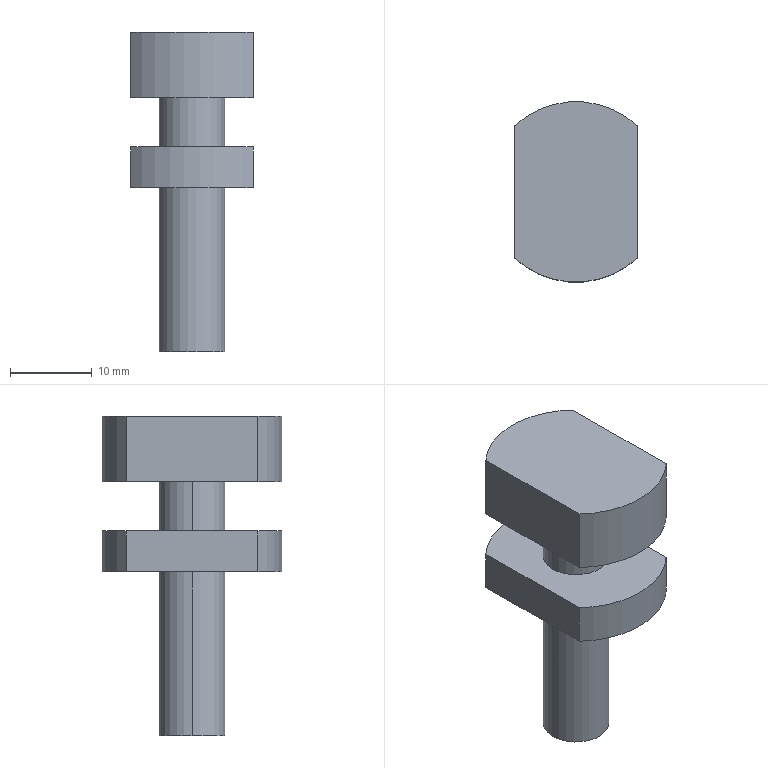Part | STEP file | iron shell displacement union | 1 solid | 17 faces | box 15 x 22 x 39 mm | volume 5236 mm3 | plane 9 | cylinder 8 | commonest cylinder face diameters 8 x4 22 x4
STEP:
#1=CARTESIAN_POINT('',(0.,0.,0.));
#2=DIRECTION('',(0.,0.,1.));
#3=DIRECTION('',(1.,0.,0.));
#4=AXIS2_PLACEMENT_3D('',#1,#2,#3);
#5=CARTESIAN_POINT('',(4.,0.,0.));
#6=VERTEX_POINT('',#5);
#7=CARTESIAN_POINT('',(-4.,0.,0.));
#8=VERTEX_POINT('',#7);
#9=CARTESIAN_POINT('',(0.,0.,0.));
#10=DIRECTION('',(0.,0.,1.));
#11=DIRECTION('',(1.,0.,0.));
#12=AXIS2_PLACEMENT_3D('',#9,#10,#11);
#13=CIRCLE('',#12,4.);
#14=CARTESIAN_POINT('',(0.,0.,39.));
#15=DIRECTION('',(0.,0.,1.));
#16=DIRECTION('',(1.,0.,0.));
#17=AXIS2_PLACEMENT_3D('',#14,#15,#16);
#18=CYLINDRICAL_SURFACE('',#17,4.);
#19=CARTESIAN_POINT('',(0.,-39.));
#20=DIRECTION('',(1.,0.));
#21=VECTOR('',#20,1.);
#22=LINE('',#19,#21);
#23=(GEOMETRIC_REPRESENTATION_CONTEXT(2)PARAMETRIC_REPRESENTATION_CONTEXT()REPRESENTATION_CONTEXT('',''));
#24=DEFINITIONAL_REPRESENTATION('',(#22),#23);
#25=PCURVE('',#18,#24);
#26=CARTESIAN_POINT('',(0.,0.,0.));
#27=DIRECTION('',(0.,0.,1.));
#28=DIRECTION('',(1.,0.,0.));
#29=AXIS2_PLACEMENT_3D('',#26,#27,#28);
#30=PLANE('',#29);
#31=CARTESIAN_POINT('',(0.,0.));
#32=DIRECTION('',(1.,0.));
#33=AXIS2_PLACEMENT_2D('',#31,#32);
#34=CIRCLE('',#33,4.);
#35=(GEOMETRIC_REPRESENTATION_CONTEXT(2)PARAMETRIC_REPRESENTATION_CONTEXT()REPRESENTATION_CONTEXT('',''));
#36=DEFINITIONAL_REPRESENTATION('',(#34),#35);
#37=PCURVE('',#30,#36);
#38=SURFACE_CURVE('',#13,(#25,#37),.PCURVE_S1.);
#39=EDGE_CURVE('',#6,#8,#38,.T.);
#40=ORIENTED_EDGE('',*,*,#39,.T.);
#41=CARTESIAN_POINT('',(-4.,0.,20.));
#42=VERTEX_POINT('',#41);
#43=CARTESIAN_POINT('',(-4.,0.,39.));
#44=DIRECTION('',(0.,0.,1.));
#45=VECTOR('',#44,1.);
#46=LINE('',#43,#45);
#47=CARTESIAN_POINT('',(3.142,0.));
#48=DIRECTION('',(0.,1.));
#49=VECTOR('',#48,1.);
#50=LINE('',#47,#49);
#51=(GEOMETRIC_REPRESENTATION_CONTEXT(2)PARAMETRIC_REPRESENTATION_CONTEXT()REPRESENTATION_CONTEXT('',''));
#52=DEFINITIONAL_REPRESENTATION('',(#50),#51);
#53=PCURVE('',#18,#52);
#54=CARTESIAN_POINT('',(0.,0.,39.));
#55=DIRECTION('',(0.,0.,1.));
#56=DIRECTION('',(1.,0.,0.));
#57=AXIS2_PLACEMENT_3D('',#54,#55,#56);
#58=CYLINDRICAL_SURFACE('',#57,4.);
#59=CARTESIAN_POINT('',(3.142,0.));
#60=DIRECTION('',(0.,1.));
#61=VECTOR('',#60,1.);
#62=LINE('',#59,#61);
#63=(GEOMETRIC_REPRESENTATION_CONTEXT(2)PARAMETRIC_REPRESENTATION_CONTEXT()REPRESENTATION_CONTEXT('',''));
#64=DEFINITIONAL_REPRESENTATION('',(#62),#63);
#65=PCURVE('',#58,#64);
#66=SURFACE_CURVE('',#46,(#53,#65),.PCURVE_S1.);
#67=EDGE_CURVE('',#8,#42,#66,.T.);
#68=ORIENTED_EDGE('',*,*,#67,.T.);
#69=CARTESIAN_POINT('',(4.,0.,20.));
#70=VERTEX_POINT('',#69);
#71=CARTESIAN_POINT('',(0.,0.,20.));
#72=DIRECTION('',(0.,0.,1.));
#73=DIRECTION('',(1.,0.,0.));
#74=AXIS2_PLACEMENT_3D('',#71,#72,#73);
#75=CIRCLE('',#74,4.);
#76=CARTESIAN_POINT('',(0.,-19.));
#77=DIRECTION('',(1.,0.));
#78=VECTOR('',#77,1.);
#79=LINE('',#76,#78);
#80=(GEOMETRIC_REPRESENTATION_CONTEXT(2)PARAMETRIC_REPRESENTATION_CONTEXT()REPRESENTATION_CONTEXT('',''));
#81=DEFINITIONAL_REPRESENTATION('',(#79),#80);
#82=PCURVE('',#18,#81);
#83=CARTESIAN_POINT('',(-4.,0.,20.));
#84=DIRECTION('',(0.,0.,-1.));
#85=DIRECTION('',(-1.,0.,0.));
#86=AXIS2_PLACEMENT_3D('',#83,#84,#85);
#87=PLANE('',#86);
#88=CARTESIAN_POINT('',(-8.,0.));
#89=CARTESIAN_POINT('',(-8.,6.928));
#90=CARTESIAN_POINT('',(-2.,3.464));
#91=CARTESIAN_POINT('',(4.,0.));
#92=CARTESIAN_POINT('',(-2.,-3.464));
#93=CARTESIAN_POINT('',(-8.,-6.928));
#94=CARTESIAN_POINT('',(-8.,0.));
#95=(BOUNDED_CURVE()B_SPLINE_CURVE(2,(#88,#89,#90,#91,#92,#93,#94),.UNSPECIFIED.,.T.,.F.)B_SPLINE_CURVE_WITH_KNOTS((1,2,2,2,2,1),(-2.094,0.,2.094,4.189,6.283,8.378),.UNSPECIFIED.)CURVE()GEOMETRIC_REPRESENTATION_ITEM()RATIONAL_B_SPLINE_CURVE((1.,0.5,1.,0.5,1.,0.5,1.))REPRESENTATION_ITEM(''));
#96=(GEOMETRIC_REPRESENTATION_CONTEXT(2)PARAMETRIC_REPRESENTATION_CONTEXT()REPRESENTATION_CONTEXT('',''));
#97=DEFINITIONAL_REPRESENTATION('',(#95),#96);
#98=PCURVE('',#87,#97);
#99=SURFACE_CURVE('',#75,(#82,#98),.PCURVE_S1.);
#100=EDGE_CURVE('',#70,#42,#99,.T.);
#101=ORIENTED_EDGE('',*,*,#100,.F.);
#102=CARTESIAN_POINT('',(4.,0.,39.));
#103=DIRECTION('',(0.,0.,1.));
#104=VECTOR('',#103,1.);
#105=LINE('',#102,#104);
#106=CARTESIAN_POINT('',(0.,0.));
#107=DIRECTION('',(0.,1.));
#108=VECTOR('',#107,1.);
#109=LINE('',#106,#108);
#110=(GEOMETRIC_REPRESENTATION_CONTEXT(2)PARAMETRIC_REPRESENTATION_CONTEXT()REPRESENTATION_CONTEXT('',''));
#111=DEFINITIONAL_REPRESENTATION('',(#109),#110);
#112=PCURVE('',#18,#111);
#113=CARTESIAN_POINT('',(6.283,0.));
#114=DIRECTION('',(0.,1.));
#115=VECTOR('',#114,1.);
#116=LINE('',#113,#115);
#117=(GEOMETRIC_REPRESENTATION_CONTEXT(2)PARAMETRIC_REPRESENTATION_CONTEXT()REPRESENTATION_CONTEXT('',''));
#118=DEFINITIONAL_REPRESENTATION('',(#116),#117);
#119=PCURVE('',#58,#118);
#120=SURFACE_CURVE('',#105,(#112,#119),.PCURVE_S1.);
#121=EDGE_CURVE('',#6,#70,#120,.T.);
#122=ORIENTED_EDGE('',*,*,#121,.F.);
#123=EDGE_LOOP('',(#40,#68,#101,#122));
#124=FACE_BOUND('',#123,.T.);
#125=ADVANCED_FACE('',(#124),#18,.T.);
#126=CARTESIAN_POINT('',(4.,0.,25.));
#127=VERTEX_POINT('',#126);
#128=CARTESIAN_POINT('',(-4.,0.,25.));
#129=VERTEX_POINT('',#128);
#130=CARTESIAN_POINT('',(0.,0.,25.));
#131=DIRECTION('',(0.,0.,1.));
#132=DIRECTION('',(1.,0.,0.));
#133=AXIS2_PLACEMENT_3D('',#130,#131,#132);
#134=CIRCLE('',#133,4.);
#135=CARTESIAN_POINT('',(0.,0.,39.));
#136=DIRECTION('',(0.,0.,1.));
#137=DIRECTION('',(1.,0.,0.));
#138=AXIS2_PLACEMENT_3D('',#135,#136,#137);
#139=CYLINDRICAL_SURFACE('',#138,4.);
#140=CARTESIAN_POINT('',(0.,-14.));
#141=DIRECTION('',(1.,0.));
#142=VECTOR('',#141,1.);
#143=LINE('',#140,#142);
#144=(GEOMETRIC_REPRESENTATION_CONTEXT(2)PARAMETRIC_REPRESENTATION_CONTEXT()REPRESENTATION_CONTEXT('',''));
#145=DEFINITIONAL_REPRESENTATION('',(#143),#144);
#146=PCURVE('',#139,#145);
#147=CARTESIAN_POINT('',(-18.905,0.,25.));
#148=DIRECTION('',(0.,0.,1.));
#149=DIRECTION('',(1.,0.,0.));
#150=AXIS2_PLACEMENT_3D('',#147,#148,#149);
#151=PLANE('',#150);
#152=CARTESIAN_POINT('',(18.905,0.));
#153=DIRECTION('',(1.,0.));
#154=AXIS2_PLACEMENT_2D('',#152,#153);
#155=CIRCLE('',#154,4.);
#156=(GEOMETRIC_REPRESENTATION_CONTEXT(2)PARAMETRIC_REPRESENTATION_CONTEXT()REPRESENTATION_CONTEXT('',''));
#157=DEFINITIONAL_REPRESENTATION('',(#155),#156);
#158=PCURVE('',#151,#157);
#159=SURFACE_CURVE('',#134,(#146,#158),.PCURVE_S1.);
#160=EDGE_CURVE('',#127,#129,#159,.T.);
#161=ORIENTED_EDGE('',*,*,#160,.T.);
#162=CARTESIAN_POINT('',(-4.,0.,31.));
#163=VERTEX_POINT('',#162);
#164=CARTESIAN_POINT('',(-4.,0.,39.));
#165=DIRECTION('',(0.,0.,1.));
#166=VECTOR('',#165,1.);
#167=LINE('',#164,#166);
#168=CARTESIAN_POINT('',(3.142,0.));
#169=DIRECTION('',(0.,1.));
#170=VECTOR('',#169,1.);
#171=LINE('',#168,#170);
#172=(GEOMETRIC_REPRESENTATION_CONTEXT(2)PARAMETRIC_REPRESENTATION_CONTEXT()REPRESENTATION_CONTEXT('',''));
#173=DEFINITIONAL_REPRESENTATION('',(#171),#172);
#174=PCURVE('',#139,#173);
#175=CARTESIAN_POINT('',(0.,0.,39.));
#176=DIRECTION('',(0.,0.,1.));
#177=DIRECTION('',(1.,0.,0.));
#178=AXIS2_PLACEMENT_3D('',#175,#176,#177);
#179=CYLINDRICAL_SURFACE('',#178,4.);
#180=CARTESIAN_POINT('',(3.142,0.));
#181=DIRECTION('',(0.,1.));
#182=VECTOR('',#181,1.);
#183=LINE('',#180,#182);
#184=(GEOMETRIC_REPRESENTATION_CONTEXT(2)PARAMETRIC_REPRESENTATION_CONTEXT()REPRESENTATION_CONTEXT('',''));
#185=DEFINITIONAL_REPRESENTATION('',(#183),#184);
#186=PCURVE('',#179,#185);
#187=SURFACE_CURVE('',#167,(#174,#186),.PCURVE_S1.);
#188=EDGE_CURVE('',#129,#163,#187,.T.);
#189=ORIENTED_EDGE('',*,*,#188,.T.);
#190=CARTESIAN_POINT('',(4.,0.,31.));
#191=VERTEX_POINT('',#190);
#192=CARTESIAN_POINT('',(0.,0.,31.));
#193=DIRECTION('',(0.,0.,1.));
#194=DIRECTION('',(1.,0.,0.));
#195=AXIS2_PLACEMENT_3D('',#192,#193,#194);
#196=CIRCLE('',#195,4.);
#197=CARTESIAN_POINT('',(0.,-8.));
#198=DIRECTION('',(1.,0.));
#199=VECTOR('',#198,1.);
#200=LINE('',#197,#199);
#201=(GEOMETRIC_REPRESENTATION_CONTEXT(2)PARAMETRIC_REPRESENTATION_CONTEXT()REPRESENTATION_CONTEXT('',''));
#202=DEFINITIONAL_REPRESENTATION('',(#200),#201);
#203=PCURVE('',#139,#202);
#204=CARTESIAN_POINT('',(-18.905,0.,31.));
#205=DIRECTION('',(0.,0.,-1.));
#206=DIRECTION('',(-1.,0.,0.));
#207=AXIS2_PLACEMENT_3D('',#204,#205,#206);
#208=PLANE('',#207);
#209=CARTESIAN_POINT('',(-22.905,0.));
#210=CARTESIAN_POINT('',(-22.905,6.928));
#211=CARTESIAN_POINT('',(-16.905,3.464));
#212=CARTESIAN_POINT('',(-10.905,0.));
#213=CARTESIAN_POINT('',(-16.905,-3.464));
#214=CARTESIAN_POINT('',(-22.905,-6.928));
#215=CARTESIAN_POINT('',(-22.905,0.));
#216=(BOUNDED_CURVE()B_SPLINE_CURVE(2,(#209,#210,#211,#212,#213,#214,#215),.UNSPECIFIED.,.T.,.F.)B_SPLINE_CURVE_WITH_KNOTS((1,2,2,2,2,1),(-2.094,0.,2.094,4.189,6.283,8.378),.UNSPECIFIED.)CURVE()GEOMETRIC_REPRESENTATION_ITEM()RATIONAL_B_SPLINE_CURVE((1.,0.5,1.,0.5,1.,0.5,1.))REPRESENTATION_ITEM(''));
#217=(GEOMETRIC_REPRESENTATION_CONTEXT(2)PARAMETRIC_REPRESENTATION_CONTEXT()REPRESENTATION_CONTEXT('',''));
#218=DEFINITIONAL_REPRESENTATION('',(#216),#217);
#219=PCURVE('',#208,#218);
#220=SURFACE_CURVE('',#196,(#203,#219),.PCURVE_S1.);
#221=EDGE_CURVE('',#191,#163,#220,.T.);
#222=ORIENTED_EDGE('',*,*,#221,.F.);
#223=CARTESIAN_POINT('',(4.,0.,39.));
#224=DIRECTION('',(0.,0.,1.));
#225=VECTOR('',#224,1.);
#226=LINE('',#223,#225);
#227=CARTESIAN_POINT('',(0.,0.));
#228=DIRECTION('',(0.,1.));
#229=VECTOR('',#228,1.);
#230=LINE('',#227,#229);
#231=(GEOMETRIC_REPRESENTATION_CONTEXT(2)PARAMETRIC_REPRESENTATION_CONTEXT()REPRESENTATION_CONTEXT('',''));
#232=DEFINITIONAL_REPRESENTATION('',(#230),#231);
#233=PCURVE('',#139,#232);
#234=CARTESIAN_POINT('',(6.283,0.));
#235=DIRECTION('',(0.,1.));
#236=VECTOR('',#235,1.);
#237=LINE('',#234,#236);
#238=(GEOMETRIC_REPRESENTATION_CONTEXT(2)PARAMETRIC_REPRESENTATION_CONTEXT()REPRESENTATION_CONTEXT('',''));
#239=DEFINITIONAL_REPRESENTATION('',(#237),#238);
#240=PCURVE('',#179,#239);
#241=SURFACE_CURVE('',#226,(#233,#240),.PCURVE_S1.);
#242=EDGE_CURVE('',#127,#191,#241,.T.);
#243=ORIENTED_EDGE('',*,*,#242,.F.);
#244=EDGE_LOOP('',(#161,#189,#222,#243));
#245=FACE_BOUND('',#244,.T.);
#246=ADVANCED_FACE('',(#245),#139,.T.);
#247=CARTESIAN_POINT('',(-7.5,-8.047,20.));
#248=VERTEX_POINT('',#247);
#249=CARTESIAN_POINT('',(-7.5,8.047,20.));
#250=VERTEX_POINT('',#249);
#251=CARTESIAN_POINT('',(-7.5,8.047,20.));
#252=DIRECTION('',(0.,1.,0.));
#253=VECTOR('',#252,1.);
#254=LINE('',#251,#253);
#255=CARTESIAN_POINT('',(-7.5,8.047,39.));
#256=DIRECTION('',(1.,0.,0.));
#257=DIRECTION('',(0.,0.,-1.));
#258=AXIS2_PLACEMENT_3D('',#255,#256,#257);
#259=PLANE('',#258);
#260=CARTESIAN_POINT('',(19.,0.));
#261=DIRECTION('',(0.,1.));
#262=VECTOR('',#261,1.);
#263=LINE('',#260,#262);
#264=(GEOMETRIC_REPRESENTATION_CONTEXT(2)PARAMETRIC_REPRESENTATION_CONTEXT()REPRESENTATION_CONTEXT('',''));
#265=DEFINITIONAL_REPRESENTATION('',(#263),#264);
#266=PCURVE('',#259,#265);
#267=CARTESIAN_POINT('',(3.5,8.047));
#268=DIRECTION('',(0.,1.));
#269=VECTOR('',#268,1.);
#270=LINE('',#267,#269);
#271=(GEOMETRIC_REPRESENTATION_CONTEXT(2)PARAMETRIC_REPRESENTATION_CONTEXT()REPRESENTATION_CONTEXT('',''));
#272=DEFINITIONAL_REPRESENTATION('',(#270),#271);
#273=PCURVE('',#87,#272);
#274=SURFACE_CURVE('',#254,(#266,#273),.PCURVE_S1.);
#275=EDGE_CURVE('',#248,#250,#274,.T.);
#276=ORIENTED_EDGE('',*,*,#275,.F.);
#277=CARTESIAN_POINT('',(-7.5,-8.047,25.));
#278=VERTEX_POINT('',#277);
#279=CARTESIAN_POINT('',(-7.5,-8.047,39.));
#280=DIRECTION('',(0.,0.,-1.));
#281=VECTOR('',#280,1.);
#282=LINE('',#279,#281);
#283=CARTESIAN_POINT('',(0.,-16.093));
#284=DIRECTION('',(1.,0.));
#285=VECTOR('',#284,1.);
#286=LINE('',#283,#285);
#287=(GEOMETRIC_REPRESENTATION_CONTEXT(2)PARAMETRIC_REPRESENTATION_CONTEXT()REPRESENTATION_CONTEXT('',''));
#288=DEFINITIONAL_REPRESENTATION('',(#286),#287);
#289=PCURVE('',#259,#288);
#290=CARTESIAN_POINT('',(0.,0.,39.));
#291=DIRECTION('',(0.,0.,-1.));
#292=DIRECTION('',(-1.,0.,0.));
#293=AXIS2_PLACEMENT_3D('',#290,#291,#292);
#294=CYLINDRICAL_SURFACE('',#293,11.);
#295=CARTESIAN_POINT('',(5.463,0.));
#296=DIRECTION('',(0.,1.));
#297=VECTOR('',#296,1.);
#298=LINE('',#295,#297);
#299=(GEOMETRIC_REPRESENTATION_CONTEXT(2)PARAMETRIC_REPRESENTATION_CONTEXT()REPRESENTATION_CONTEXT('',''));
#300=DEFINITIONAL_REPRESENTATION('',(#298),#299);
#301=PCURVE('',#294,#300);
#302=SURFACE_CURVE('',#282,(#289,#301),.PCURVE_S1.);
#303=EDGE_CURVE('',#278,#248,#302,.T.);
#304=ORIENTED_EDGE('',*,*,#303,.F.);
#305=CARTESIAN_POINT('',(-7.5,8.047,25.));
#306=VERTEX_POINT('',#305);
#307=CARTESIAN_POINT('',(-7.5,8.047,25.));
#308=DIRECTION('',(0.,-1.,0.));
#309=VECTOR('',#308,1.);
#310=LINE('',#307,#309);
#311=CARTESIAN_POINT('',(14.,0.));
#312=DIRECTION('',(0.,-1.));
#313=VECTOR('',#312,1.);
#314=LINE('',#311,#313);
#315=(GEOMETRIC_REPRESENTATION_CONTEXT(2)PARAMETRIC_REPRESENTATION_CONTEXT()REPRESENTATION_CONTEXT('',''));
#316=DEFINITIONAL_REPRESENTATION('',(#314),#315);
#317=PCURVE('',#259,#316);
#318=CARTESIAN_POINT('',(11.405,8.047));
#319=DIRECTION('',(0.,-1.));
#320=VECTOR('',#319,1.);
#321=LINE('',#318,#320);
#322=(GEOMETRIC_REPRESENTATION_CONTEXT(2)PARAMETRIC_REPRESENTATION_CONTEXT()REPRESENTATION_CONTEXT('',''));
#323=DEFINITIONAL_REPRESENTATION('',(#321),#322);
#324=PCURVE('',#151,#323);
#325=SURFACE_CURVE('',#310,(#317,#324),.PCURVE_S1.);
#326=EDGE_CURVE('',#306,#278,#325,.T.);
#327=ORIENTED_EDGE('',*,*,#326,.F.);
#328=CARTESIAN_POINT('',(-7.5,8.047,39.));
#329=DIRECTION('',(0.,0.,-1.));
#330=VECTOR('',#329,1.);
#331=LINE('',#328,#330);
#332=CARTESIAN_POINT('',(0.,0.));
#333=DIRECTION('',(1.,0.));
#334=VECTOR('',#333,1.);
#335=LINE('',#332,#334);
#336=(GEOMETRIC_REPRESENTATION_CONTEXT(2)PARAMETRIC_REPRESENTATION_CONTEXT()REPRESENTATION_CONTEXT('',''));
#337=DEFINITIONAL_REPRESENTATION('',(#335),#336);
#338=PCURVE('',#259,#337);
#339=CARTESIAN_POINT('',(0.,0.,39.));
#340=DIRECTION('',(0.,0.,-1.));
#341=DIRECTION('',(-1.,0.,0.));
#342=AXIS2_PLACEMENT_3D('',#339,#340,#341);
#343=CYLINDRICAL_SURFACE('',#342,11.);
#344=CARTESIAN_POINT('',(0.8206,0.));
#345=DIRECTION('',(0.,1.));
#346=VECTOR('',#345,1.);
#347=LINE('',#344,#346);
#348=(GEOMETRIC_REPRESENTATION_CONTEXT(2)PARAMETRIC_REPRESENTATION_CONTEXT()REPRESENTATION_CONTEXT('',''));
#349=DEFINITIONAL_REPRESENTATION('',(#347),#348);
#350=PCURVE('',#343,#349);
#351=SURFACE_CURVE('',#331,(#338,#350),.PCURVE_S1.);
#352=EDGE_CURVE('',#306,#250,#351,.T.);
#353=ORIENTED_EDGE('',*,*,#352,.T.);
#354=EDGE_LOOP('',(#276,#304,#327,#353));
#355=FACE_BOUND('',#354,.T.);
#356=ADVANCED_FACE('',(#355),#259,.F.);
#357=CARTESIAN_POINT('',(7.5,8.047,20.));
#358=VERTEX_POINT('',#357);
#359=CARTESIAN_POINT('',(0.,0.,20.));
#360=DIRECTION('',(0.,0.,-1.));
#361=DIRECTION('',(-1.,0.,0.));
#362=AXIS2_PLACEMENT_3D('',#359,#360,#361);
#363=CIRCLE('',#362,11.);
#364=CARTESIAN_POINT('',(0.,19.));
#365=DIRECTION('',(1.,0.));
#366=VECTOR('',#365,1.);
#367=LINE('',#364,#366);
#368=(GEOMETRIC_REPRESENTATION_CONTEXT(2)PARAMETRIC_REPRESENTATION_CONTEXT()REPRESENTATION_CONTEXT('',''));
#369=DEFINITIONAL_REPRESENTATION('',(#367),#368);
#370=PCURVE('',#343,#369);
#371=CARTESIAN_POINT('',(-4.,0.));
#372=DIRECTION('',(1.,0.));
#373=AXIS2_PLACEMENT_2D('',#371,#372);
#374=CIRCLE('',#373,11.);
#375=(GEOMETRIC_REPRESENTATION_CONTEXT(2)PARAMETRIC_REPRESENTATION_CONTEXT()REPRESENTATION_CONTEXT('',''));
#376=DEFINITIONAL_REPRESENTATION('',(#374),#375);
#377=PCURVE('',#87,#376);
#378=SURFACE_CURVE('',#363,(#370,#377),.PCURVE_S1.);
#379=EDGE_CURVE('',#250,#358,#378,.T.);
#380=ORIENTED_EDGE('',*,*,#379,.F.);
#381=ORIENTED_EDGE('',*,*,#352,.F.);
#382=CARTESIAN_POINT('',(7.5,8.047,25.));
#383=VERTEX_POINT('',#382);
#384=CARTESIAN_POINT('',(0.,0.,25.));
#385=DIRECTION('',(0.,0.,1.));
#386=DIRECTION('',(1.,0.,0.));
#387=AXIS2_PLACEMENT_3D('',#384,#385,#386);
#388=CIRCLE('',#387,11.);
#389=CARTESIAN_POINT('',(3.142,14.));
#390=DIRECTION('',(-1.,0.));
#391=VECTOR('',#390,1.);
#392=LINE('',#389,#391);
#393=(GEOMETRIC_REPRESENTATION_CONTEXT(2)PARAMETRIC_REPRESENTATION_CONTEXT()REPRESENTATION_CONTEXT('',''));
#394=DEFINITIONAL_REPRESENTATION('',(#392),#393);
#395=PCURVE('',#343,#394);
#396=CARTESIAN_POINT('',(18.905,0.));
#397=DIRECTION('',(1.,0.));
#398=AXIS2_PLACEMENT_2D('',#396,#397);
#399=CIRCLE('',#398,11.);
#400=(GEOMETRIC_REPRESENTATION_CONTEXT(2)PARAMETRIC_REPRESENTATION_CONTEXT()REPRESENTATION_CONTEXT('',''));
#401=DEFINITIONAL_REPRESENTATION('',(#399),#400);
#402=PCURVE('',#151,#401);
#403=SURFACE_CURVE('',#388,(#395,#402),.PCURVE_S1.);
#404=EDGE_CURVE('',#383,#306,#403,.T.);
#405=ORIENTED_EDGE('',*,*,#404,.F.);
#406=CARTESIAN_POINT('',(7.5,8.047,39.));
#407=DIRECTION('',(0.,0.,-1.));
#408=VECTOR('',#407,1.);
#409=LINE('',#406,#408);
#410=CARTESIAN_POINT('',(2.321,0.));
#411=DIRECTION('',(0.,1.));
#412=VECTOR('',#411,1.);
#413=LINE('',#410,#412);
#414=(GEOMETRIC_REPRESENTATION_CONTEXT(2)PARAMETRIC_REPRESENTATION_CONTEXT()REPRESENTATION_CONTEXT('',''));
#415=DEFINITIONAL_REPRESENTATION('',(#413),#414);
#416=PCURVE('',#343,#415);
#417=CARTESIAN_POINT('',(7.5,8.047,39.));
#418=DIRECTION('',(-1.,0.,0.));
#419=DIRECTION('',(0.,0.,1.));
#420=AXIS2_PLACEMENT_3D('',#417,#418,#419);
#421=PLANE('',#420);
#422=CARTESIAN_POINT('',(0.,0.));
#423=DIRECTION('',(-1.,0.));
#424=VECTOR('',#423,1.);
#425=LINE('',#422,#424);
#426=(GEOMETRIC_REPRESENTATION_CONTEXT(2)PARAMETRIC_REPRESENTATION_CONTEXT()REPRESENTATION_CONTEXT('',''));
#427=DEFINITIONAL_REPRESENTATION('',(#425),#426);
#428=PCURVE('',#421,#427);
#429=SURFACE_CURVE('',#409,(#416,#428),.PCURVE_S1.);
#430=EDGE_CURVE('',#383,#358,#429,.T.);
#431=ORIENTED_EDGE('',*,*,#430,.T.);
#432=EDGE_LOOP('',(#380,#381,#405,#431));
#433=FACE_BOUND('',#432,.T.);
#434=ADVANCED_FACE('',(#433),#343,.T.);
#435=CARTESIAN_POINT('',(7.5,-8.047,20.));
#436=VERTEX_POINT('',#435);
#437=CARTESIAN_POINT('',(7.5,8.047,20.));
#438=DIRECTION('',(0.,-1.,0.));
#439=VECTOR('',#438,1.);
#440=LINE('',#437,#439);
#441=CARTESIAN_POINT('',(-19.,0.));
#442=DIRECTION('',(0.,-1.));
#443=VECTOR('',#442,1.);
#444=LINE('',#441,#443);
#445=(GEOMETRIC_REPRESENTATION_CONTEXT(2)PARAMETRIC_REPRESENTATION_CONTEXT()REPRESENTATION_CONTEXT('',''));
#446=DEFINITIONAL_REPRESENTATION('',(#444),#445);
#447=PCURVE('',#421,#446);
#448=CARTESIAN_POINT('',(-11.5,8.047));
#449=DIRECTION('',(0.,-1.));
#450=VECTOR('',#449,1.);
#451=LINE('',#448,#450);
#452=(GEOMETRIC_REPRESENTATION_CONTEXT(2)PARAMETRIC_REPRESENTATION_CONTEXT()REPRESENTATION_CONTEXT('',''));
#453=DEFINITIONAL_REPRESENTATION('',(#451),#452);
#454=PCURVE('',#87,#453);
#455=SURFACE_CURVE('',#440,(#447,#454),.PCURVE_S1.);
#456=EDGE_CURVE('',#358,#436,#455,.T.);
#457=ORIENTED_EDGE('',*,*,#456,.F.);
#458=ORIENTED_EDGE('',*,*,#430,.F.);
#459=CARTESIAN_POINT('',(7.5,-8.047,25.));
#460=VERTEX_POINT('',#459);
#461=CARTESIAN_POINT('',(7.5,8.047,25.));
#462=DIRECTION('',(0.,1.,0.));
#463=VECTOR('',#462,1.);
#464=LINE('',#461,#463);
#465=CARTESIAN_POINT('',(-14.,0.));
#466=DIRECTION('',(0.,1.));
#467=VECTOR('',#466,1.);
#468=LINE('',#465,#467);
#469=(GEOMETRIC_REPRESENTATION_CONTEXT(2)PARAMETRIC_REPRESENTATION_CONTEXT()REPRESENTATION_CONTEXT('',''));
#470=DEFINITIONAL_REPRESENTATION('',(#468),#469);
#471=PCURVE('',#421,#470);
#472=CARTESIAN_POINT('',(26.405,8.047));
#473=DIRECTION('',(0.,1.));
#474=VECTOR('',#473,1.);
#475=LINE('',#472,#474);
#476=(GEOMETRIC_REPRESENTATION_CONTEXT(2)PARAMETRIC_REPRESENTATION_CONTEXT()REPRESENTATION_CONTEXT('',''));
#477=DEFINITIONAL_REPRESENTATION('',(#475),#476);
#478=PCURVE('',#151,#477);
#479=SURFACE_CURVE('',#464,(#471,#478),.PCURVE_S1.);
#480=EDGE_CURVE('',#460,#383,#479,.T.);
#481=ORIENTED_EDGE('',*,*,#480,.F.);
#482=CARTESIAN_POINT('',(7.5,-8.047,39.));
#483=DIRECTION('',(0.,0.,-1.));
#484=VECTOR('',#483,1.);
#485=LINE('',#482,#484);
#486=CARTESIAN_POINT('',(0.,-16.093));
#487=DIRECTION('',(-1.,0.));
#488=VECTOR('',#487,1.);
#489=LINE('',#486,#488);
#490=(GEOMETRIC_REPRESENTATION_CONTEXT(2)PARAMETRIC_REPRESENTATION_CONTEXT()REPRESENTATION_CONTEXT('',''));
#491=DEFINITIONAL_REPRESENTATION('',(#489),#490);
#492=PCURVE('',#421,#491);
#493=CARTESIAN_POINT('',(3.962,0.));
#494=DIRECTION('',(0.,1.));
#495=VECTOR('',#494,1.);
#496=LINE('',#493,#495);
#497=(GEOMETRIC_REPRESENTATION_CONTEXT(2)PARAMETRIC_REPRESENTATION_CONTEXT()REPRESENTATION_CONTEXT('',''));
#498=DEFINITIONAL_REPRESENTATION('',(#496),#497);
#499=PCURVE('',#294,#498);
#500=SURFACE_CURVE('',#485,(#492,#499),.PCURVE_S1.);
#501=EDGE_CURVE('',#460,#436,#500,.T.);
#502=ORIENTED_EDGE('',*,*,#501,.T.);
#503=EDGE_LOOP('',(#457,#458,#481,#502));
#504=FACE_BOUND('',#503,.T.);
#505=ADVANCED_FACE('',(#504),#421,.F.);
#506=CARTESIAN_POINT('',(0.,0.,20.));
#507=DIRECTION('',(0.,0.,-1.));
#508=DIRECTION('',(-1.,0.,0.));
#509=AXIS2_PLACEMENT_3D('',#506,#507,#508);
#510=CIRCLE('',#509,11.);
#511=CARTESIAN_POINT('',(0.,19.));
#512=DIRECTION('',(1.,0.));
#513=VECTOR('',#512,1.);
#514=LINE('',#511,#513);
#515=(GEOMETRIC_REPRESENTATION_CONTEXT(2)PARAMETRIC_REPRESENTATION_CONTEXT()REPRESENTATION_CONTEXT('',''));
#516=DEFINITIONAL_REPRESENTATION('',(#514),#515);
#517=PCURVE('',#294,#516);
#518=CARTESIAN_POINT('',(-4.,0.));
#519=DIRECTION('',(1.,0.));
#520=AXIS2_PLACEMENT_2D('',#518,#519);
#521=CIRCLE('',#520,11.);
#522=(GEOMETRIC_REPRESENTATION_CONTEXT(2)PARAMETRIC_REPRESENTATION_CONTEXT()REPRESENTATION_CONTEXT('',''));
#523=DEFINITIONAL_REPRESENTATION('',(#521),#522);
#524=PCURVE('',#87,#523);
#525=SURFACE_CURVE('',#510,(#517,#524),.PCURVE_S1.);
#526=EDGE_CURVE('',#436,#248,#525,.T.);
#527=ORIENTED_EDGE('',*,*,#526,.F.);
#528=ORIENTED_EDGE('',*,*,#501,.F.);
#529=CARTESIAN_POINT('',(0.,0.,25.));
#530=DIRECTION('',(0.,0.,1.));
#531=DIRECTION('',(1.,0.,0.));
#532=AXIS2_PLACEMENT_3D('',#529,#530,#531);
#533=CIRCLE('',#532,11.);
#534=CARTESIAN_POINT('',(9.425,14.));
#535=DIRECTION('',(-1.,0.));
#536=VECTOR('',#535,1.);
#537=LINE('',#534,#536);
#538=(GEOMETRIC_REPRESENTATION_CONTEXT(2)PARAMETRIC_REPRESENTATION_CONTEXT()REPRESENTATION_CONTEXT('',''));
#539=DEFINITIONAL_REPRESENTATION('',(#537),#538);
#540=PCURVE('',#294,#539);
#541=CARTESIAN_POINT('',(18.905,0.));
#542=DIRECTION('',(1.,0.));
#543=AXIS2_PLACEMENT_2D('',#541,#542);
#544=CIRCLE('',#543,11.);
#545=(GEOMETRIC_REPRESENTATION_CONTEXT(2)PARAMETRIC_REPRESENTATION_CONTEXT()REPRESENTATION_CONTEXT('',''));
#546=DEFINITIONAL_REPRESENTATION('',(#544),#545);
#547=PCURVE('',#151,#546);
#548=SURFACE_CURVE('',#533,(#540,#547),.PCURVE_S1.);
#549=EDGE_CURVE('',#278,#460,#548,.T.);
#550=ORIENTED_EDGE('',*,*,#549,.F.);
#551=ORIENTED_EDGE('',*,*,#303,.T.);
#552=EDGE_LOOP('',(#527,#528,#550,#551));
#553=FACE_BOUND('',#552,.T.);
#554=ADVANCED_FACE('',(#553),#294,.T.);
#555=CARTESIAN_POINT('',(7.5,-8.047,31.));
#556=VERTEX_POINT('',#555);
#557=CARTESIAN_POINT('',(-7.5,-8.047,31.));
#558=VERTEX_POINT('',#557);
#559=CARTESIAN_POINT('',(0.,0.,31.));
#560=DIRECTION('',(0.,0.,-1.));
#561=DIRECTION('',(-1.,0.,0.));
#562=AXIS2_PLACEMENT_3D('',#559,#560,#561);
#563=CIRCLE('',#562,11.);
#564=CARTESIAN_POINT('',(0.,0.,39.));
#565=DIRECTION('',(0.,0.,-1.));
#566=DIRECTION('',(-1.,0.,0.));
#567=AXIS2_PLACEMENT_3D('',#564,#565,#566);
#568=CYLINDRICAL_SURFACE('',#567,11.);
#569=CARTESIAN_POINT('',(0.,8.));
#570=DIRECTION('',(1.,0.));
#571=VECTOR('',#570,1.);
#572=LINE('',#569,#571);
#573=(GEOMETRIC_REPRESENTATION_CONTEXT(2)PARAMETRIC_REPRESENTATION_CONTEXT()REPRESENTATION_CONTEXT('',''));
#574=DEFINITIONAL_REPRESENTATION('',(#572),#573);
#575=PCURVE('',#568,#574);
#576=CARTESIAN_POINT('',(-18.905,0.));
#577=DIRECTION('',(1.,0.));
#578=AXIS2_PLACEMENT_2D('',#576,#577);
#579=CIRCLE('',#578,11.);
#580=(GEOMETRIC_REPRESENTATION_CONTEXT(2)PARAMETRIC_REPRESENTATION_CONTEXT()REPRESENTATION_CONTEXT('',''));
#581=DEFINITIONAL_REPRESENTATION('',(#579),#580);
#582=PCURVE('',#208,#581);
#583=SURFACE_CURVE('',#563,(#575,#582),.PCURVE_S1.);
#584=EDGE_CURVE('',#556,#558,#583,.T.);
#585=ORIENTED_EDGE('',*,*,#584,.F.);
#586=CARTESIAN_POINT('',(7.5,-8.047,39.));
#587=VERTEX_POINT('',#586);
#588=CARTESIAN_POINT('',(7.5,-8.047,39.));
#589=DIRECTION('',(0.,0.,-1.));
#590=VECTOR('',#589,1.);
#591=LINE('',#588,#590);
#592=CARTESIAN_POINT('',(3.962,0.));
#593=DIRECTION('',(0.,1.));
#594=VECTOR('',#593,1.);
#595=LINE('',#592,#594);
#596=(GEOMETRIC_REPRESENTATION_CONTEXT(2)PARAMETRIC_REPRESENTATION_CONTEXT()REPRESENTATION_CONTEXT('',''));
#597=DEFINITIONAL_REPRESENTATION('',(#595),#596);
#598=PCURVE('',#568,#597);
#599=CARTESIAN_POINT('',(7.5,8.047,39.));
#600=DIRECTION('',(-1.,0.,0.));
#601=DIRECTION('',(0.,0.,1.));
#602=AXIS2_PLACEMENT_3D('',#599,#600,#601);
#603=PLANE('',#602);
#604=CARTESIAN_POINT('',(0.,-16.093));
#605=DIRECTION('',(-1.,0.));
#606=VECTOR('',#605,1.);
#607=LINE('',#604,#606);
#608=(GEOMETRIC_REPRESENTATION_CONTEXT(2)PARAMETRIC_REPRESENTATION_CONTEXT()REPRESENTATION_CONTEXT('',''));
#609=DEFINITIONAL_REPRESENTATION('',(#607),#608);
#610=PCURVE('',#603,#609);
#611=SURFACE_CURVE('',#591,(#598,#610),.PCURVE_S1.);
#612=EDGE_CURVE('',#587,#556,#611,.T.);
#613=ORIENTED_EDGE('',*,*,#612,.F.);
#614=CARTESIAN_POINT('',(-7.5,-8.047,39.));
#615=VERTEX_POINT('',#614);
#616=CARTESIAN_POINT('',(0.,0.,39.));
#617=DIRECTION('',(0.,0.,1.));
#618=DIRECTION('',(1.,0.,0.));
#619=AXIS2_PLACEMENT_3D('',#616,#617,#618);
#620=CIRCLE('',#619,11.);
#621=CARTESIAN_POINT('',(9.425,0.));
#622=DIRECTION('',(-1.,0.));
#623=VECTOR('',#622,1.);
#624=LINE('',#621,#623);
#625=(GEOMETRIC_REPRESENTATION_CONTEXT(2)PARAMETRIC_REPRESENTATION_CONTEXT()REPRESENTATION_CONTEXT('',''));
#626=DEFINITIONAL_REPRESENTATION('',(#624),#625);
#627=PCURVE('',#568,#626);
#628=CARTESIAN_POINT('',(0.,0.,39.));
#629=DIRECTION('',(0.,0.,1.));
#630=DIRECTION('',(1.,0.,0.));
#631=AXIS2_PLACEMENT_3D('',#628,#629,#630);
#632=PLANE('',#631);
#633=CARTESIAN_POINT('',(0.,0.));
#634=DIRECTION('',(1.,0.));
#635=AXIS2_PLACEMENT_2D('',#633,#634);
#636=CIRCLE('',#635,11.);
#637=(GEOMETRIC_REPRESENTATION_CONTEXT(2)PARAMETRIC_REPRESENTATION_CONTEXT()REPRESENTATION_CONTEXT('',''));
#638=DEFINITIONAL_REPRESENTATION('',(#636),#637);
#639=PCURVE('',#632,#638);
#640=SURFACE_CURVE('',#620,(#627,#639),.PCURVE_S1.);
#641=EDGE_CURVE('',#615,#587,#640,.T.);
#642=ORIENTED_EDGE('',*,*,#641,.F.);
#643=CARTESIAN_POINT('',(-7.5,-8.047,39.));
#644=DIRECTION('',(0.,0.,-1.));
#645=VECTOR('',#644,1.);
#646=LINE('',#643,#645);
#647=CARTESIAN_POINT('',(5.463,0.));
#648=DIRECTION('',(0.,1.));
#649=VECTOR('',#648,1.);
#650=LINE('',#647,#649);
#651=(GEOMETRIC_REPRESENTATION_CONTEXT(2)PARAMETRIC_REPRESENTATION_CONTEXT()REPRESENTATION_CONTEXT('',''));
#652=DEFINITIONAL_REPRESENTATION('',(#650),#651);
#653=PCURVE('',#568,#652);
#654=CARTESIAN_POINT('',(-7.5,8.047,39.));
#655=DIRECTION('',(1.,0.,0.));
#656=DIRECTION('',(0.,0.,-1.));
#657=AXIS2_PLACEMENT_3D('',#654,#655,#656);
#658=PLANE('',#657);
#659=CARTESIAN_POINT('',(0.,-16.093));
#660=DIRECTION('',(1.,0.));
#661=VECTOR('',#660,1.);
#662=LINE('',#659,#661);
#663=(GEOMETRIC_REPRESENTATION_CONTEXT(2)PARAMETRIC_REPRESENTATION_CONTEXT()REPRESENTATION_CONTEXT('',''));
#664=DEFINITIONAL_REPRESENTATION('',(#662),#663);
#665=PCURVE('',#658,#664);
#666=SURFACE_CURVE('',#646,(#653,#665),.PCURVE_S1.);
#667=EDGE_CURVE('',#615,#558,#666,.T.);
#668=ORIENTED_EDGE('',*,*,#667,.T.);
#669=EDGE_LOOP('',(#585,#613,#642,#668));
#670=FACE_BOUND('',#669,.T.);
#671=ADVANCED_FACE('',(#670),#568,.T.);
#672=CARTESIAN_POINT('',(7.5,8.047,31.));
#673=VERTEX_POINT('',#672);
#674=CARTESIAN_POINT('',(7.5,8.047,31.));
#675=DIRECTION('',(0.,-1.,0.));
#676=VECTOR('',#675,1.);
#677=LINE('',#674,#676);
#678=CARTESIAN_POINT('',(-8.,0.));
#679=DIRECTION('',(0.,-1.));
#680=VECTOR('',#679,1.);
#681=LINE('',#678,#680);
#682=(GEOMETRIC_REPRESENTATION_CONTEXT(2)PARAMETRIC_REPRESENTATION_CONTEXT()REPRESENTATION_CONTEXT('',''));
#683=DEFINITIONAL_REPRESENTATION('',(#681),#682);
#684=PCURVE('',#603,#683);
#685=CARTESIAN_POINT('',(-26.405,8.047));
#686=DIRECTION('',(0.,-1.));
#687=VECTOR('',#686,1.);
#688=LINE('',#685,#687);
#689=(GEOMETRIC_REPRESENTATION_CONTEXT(2)PARAMETRIC_REPRESENTATION_CONTEXT()REPRESENTATION_CONTEXT('',''));
#690=DEFINITIONAL_REPRESENTATION('',(#688),#689);
#691=PCURVE('',#208,#690);
#692=SURFACE_CURVE('',#677,(#684,#691),.PCURVE_S1.);
#693=EDGE_CURVE('',#673,#556,#692,.T.);
#694=ORIENTED_EDGE('',*,*,#693,.F.);
#695=CARTESIAN_POINT('',(7.5,8.047,39.));
#696=VERTEX_POINT('',#695);
#697=CARTESIAN_POINT('',(7.5,8.047,39.));
#698=DIRECTION('',(0.,0.,-1.));
#699=VECTOR('',#698,1.);
#700=LINE('',#697,#699);
#701=CARTESIAN_POINT('',(0.,0.));
#702=DIRECTION('',(-1.,0.));
#703=VECTOR('',#702,1.);
#704=LINE('',#701,#703);
#705=(GEOMETRIC_REPRESENTATION_CONTEXT(2)PARAMETRIC_REPRESENTATION_CONTEXT()REPRESENTATION_CONTEXT('',''));
#706=DEFINITIONAL_REPRESENTATION('',(#704),#705);
#707=PCURVE('',#603,#706);
#708=CARTESIAN_POINT('',(0.,0.,39.));
#709=DIRECTION('',(0.,0.,-1.));
#710=DIRECTION('',(-1.,0.,0.));
#711=AXIS2_PLACEMENT_3D('',#708,#709,#710);
#712=CYLINDRICAL_SURFACE('',#711,11.);
#713=CARTESIAN_POINT('',(2.321,0.));
#714=DIRECTION('',(0.,1.));
#715=VECTOR('',#714,1.);
#716=LINE('',#713,#715);
#717=(GEOMETRIC_REPRESENTATION_CONTEXT(2)PARAMETRIC_REPRESENTATION_CONTEXT()REPRESENTATION_CONTEXT('',''));
#718=DEFINITIONAL_REPRESENTATION('',(#716),#717);
#719=PCURVE('',#712,#718);
#720=SURFACE_CURVE('',#700,(#707,#719),.PCURVE_S1.);
#721=EDGE_CURVE('',#696,#673,#720,.T.);
#722=ORIENTED_EDGE('',*,*,#721,.F.);
#723=CARTESIAN_POINT('',(7.5,8.047,39.));
#724=DIRECTION('',(0.,1.,0.));
#725=VECTOR('',#724,1.);
#726=LINE('',#723,#725);
#727=CARTESIAN_POINT('',(0.,0.));
#728=DIRECTION('',(0.,1.));
#729=VECTOR('',#728,1.);
#730=LINE('',#727,#729);
#731=(GEOMETRIC_REPRESENTATION_CONTEXT(2)PARAMETRIC_REPRESENTATION_CONTEXT()REPRESENTATION_CONTEXT('',''));
#732=DEFINITIONAL_REPRESENTATION('',(#730),#731);
#733=PCURVE('',#603,#732);
#734=CARTESIAN_POINT('',(7.5,8.047));
#735=DIRECTION('',(0.,1.));
#736=VECTOR('',#735,1.);
#737=LINE('',#734,#736);
#738=(GEOMETRIC_REPRESENTATION_CONTEXT(2)PARAMETRIC_REPRESENTATION_CONTEXT()REPRESENTATION_CONTEXT('',''));
#739=DEFINITIONAL_REPRESENTATION('',(#737),#738);
#740=PCURVE('',#632,#739);
#741=SURFACE_CURVE('',#726,(#733,#740),.PCURVE_S1.);
#742=EDGE_CURVE('',#587,#696,#741,.T.);
#743=ORIENTED_EDGE('',*,*,#742,.F.);
#744=ORIENTED_EDGE('',*,*,#612,.T.);
#745=EDGE_LOOP('',(#694,#722,#743,#744));
#746=FACE_BOUND('',#745,.T.);
#747=ADVANCED_FACE('',(#746),#603,.F.);
#748=CARTESIAN_POINT('',(-7.5,8.047,31.));
#749=VERTEX_POINT('',#748);
#750=CARTESIAN_POINT('',(0.,0.,31.));
#751=DIRECTION('',(0.,0.,-1.));
#752=DIRECTION('',(-1.,0.,0.));
#753=AXIS2_PLACEMENT_3D('',#750,#751,#752);
#754=CIRCLE('',#753,11.);
#755=CARTESIAN_POINT('',(0.,8.));
#756=DIRECTION('',(1.,0.));
#757=VECTOR('',#756,1.);
#758=LINE('',#755,#757);
#759=(GEOMETRIC_REPRESENTATION_CONTEXT(2)PARAMETRIC_REPRESENTATION_CONTEXT()REPRESENTATION_CONTEXT('',''));
#760=DEFINITIONAL_REPRESENTATION('',(#758),#759);
#761=PCURVE('',#712,#760);
#762=CARTESIAN_POINT('',(-18.905,0.));
#763=DIRECTION('',(1.,0.));
#764=AXIS2_PLACEMENT_2D('',#762,#763);
#765=CIRCLE('',#764,11.);
#766=(GEOMETRIC_REPRESENTATION_CONTEXT(2)PARAMETRIC_REPRESENTATION_CONTEXT()REPRESENTATION_CONTEXT('',''));
#767=DEFINITIONAL_REPRESENTATION('',(#765),#766);
#768=PCURVE('',#208,#767);
#769=SURFACE_CURVE('',#754,(#761,#768),.PCURVE_S1.);
#770=EDGE_CURVE('',#749,#673,#769,.T.);
#771=ORIENTED_EDGE('',*,*,#770,.F.);
#772=CARTESIAN_POINT('',(-7.5,8.047,39.));
#773=VERTEX_POINT('',#772);
#774=CARTESIAN_POINT('',(-7.5,8.047,39.));
#775=DIRECTION('',(0.,0.,-1.));
#776=VECTOR('',#775,1.);
#777=LINE('',#774,#776);
#778=CARTESIAN_POINT('',(0.8206,0.));
#779=DIRECTION('',(0.,1.));
#780=VECTOR('',#779,1.);
#781=LINE('',#778,#780);
#782=(GEOMETRIC_REPRESENTATION_CONTEXT(2)PARAMETRIC_REPRESENTATION_CONTEXT()REPRESENTATION_CONTEXT('',''));
#783=DEFINITIONAL_REPRESENTATION('',(#781),#782);
#784=PCURVE('',#712,#783);
#785=CARTESIAN_POINT('',(0.,0.));
#786=DIRECTION('',(1.,0.));
#787=VECTOR('',#786,1.);
#788=LINE('',#785,#787);
#789=(GEOMETRIC_REPRESENTATION_CONTEXT(2)PARAMETRIC_REPRESENTATION_CONTEXT()REPRESENTATION_CONTEXT('',''));
#790=DEFINITIONAL_REPRESENTATION('',(#788),#789);
#791=PCURVE('',#658,#790);
#792=SURFACE_CURVE('',#777,(#784,#791),.PCURVE_S1.);
#793=EDGE_CURVE('',#773,#749,#792,.T.);
#794=ORIENTED_EDGE('',*,*,#793,.F.);
#795=CARTESIAN_POINT('',(0.,0.,39.));
#796=DIRECTION('',(0.,0.,1.));
#797=DIRECTION('',(1.,0.,0.));
#798=AXIS2_PLACEMENT_3D('',#795,#796,#797);
#799=CIRCLE('',#798,11.);
#800=CARTESIAN_POINT('',(3.142,0.));
#801=DIRECTION('',(-1.,0.));
#802=VECTOR('',#801,1.);
#803=LINE('',#800,#802);
#804=(GEOMETRIC_REPRESENTATION_CONTEXT(2)PARAMETRIC_REPRESENTATION_CONTEXT()REPRESENTATION_CONTEXT('',''));
#805=DEFINITIONAL_REPRESENTATION('',(#803),#804);
#806=PCURVE('',#712,#805);
#807=CARTESIAN_POINT('',(0.,0.));
#808=DIRECTION('',(1.,0.));
#809=AXIS2_PLACEMENT_2D('',#807,#808);
#810=CIRCLE('',#809,11.);
#811=(GEOMETRIC_REPRESENTATION_CONTEXT(2)PARAMETRIC_REPRESENTATION_CONTEXT()REPRESENTATION_CONTEXT('',''));
#812=DEFINITIONAL_REPRESENTATION('',(#810),#811);
#813=PCURVE('',#632,#812);
#814=SURFACE_CURVE('',#799,(#806,#813),.PCURVE_S1.);
#815=EDGE_CURVE('',#696,#773,#814,.T.);
#816=ORIENTED_EDGE('',*,*,#815,.F.);
#817=ORIENTED_EDGE('',*,*,#721,.T.);
#818=EDGE_LOOP('',(#771,#794,#816,#817));
#819=FACE_BOUND('',#818,.T.);
#820=ADVANCED_FACE('',(#819),#712,.T.);
#821=CARTESIAN_POINT('',(-7.5,8.047,31.));
#822=DIRECTION('',(0.,1.,0.));
#823=VECTOR('',#822,1.);
#824=LINE('',#821,#823);
#825=CARTESIAN_POINT('',(8.,0.));
#826=DIRECTION('',(0.,1.));
#827=VECTOR('',#826,1.);
#828=LINE('',#825,#827);
#829=(GEOMETRIC_REPRESENTATION_CONTEXT(2)PARAMETRIC_REPRESENTATION_CONTEXT()REPRESENTATION_CONTEXT('',''));
#830=DEFINITIONAL_REPRESENTATION('',(#828),#829);
#831=PCURVE('',#658,#830);
#832=CARTESIAN_POINT('',(-11.405,8.047));
#833=DIRECTION('',(0.,1.));
#834=VECTOR('',#833,1.);
#835=LINE('',#832,#834);
#836=(GEOMETRIC_REPRESENTATION_CONTEXT(2)PARAMETRIC_REPRESENTATION_CONTEXT()REPRESENTATION_CONTEXT('',''));
#837=DEFINITIONAL_REPRESENTATION('',(#835),#836);
#838=PCURVE('',#208,#837);
#839=SURFACE_CURVE('',#824,(#831,#838),.PCURVE_S1.);
#840=EDGE_CURVE('',#558,#749,#839,.T.);
#841=ORIENTED_EDGE('',*,*,#840,.F.);
#842=ORIENTED_EDGE('',*,*,#667,.F.);
#843=CARTESIAN_POINT('',(-7.5,8.047,39.));
#844=DIRECTION('',(0.,-1.,0.));
#845=VECTOR('',#844,1.);
#846=LINE('',#843,#845);
#847=CARTESIAN_POINT('',(0.,0.));
#848=DIRECTION('',(0.,-1.));
#849=VECTOR('',#848,1.);
#850=LINE('',#847,#849);
#851=(GEOMETRIC_REPRESENTATION_CONTEXT(2)PARAMETRIC_REPRESENTATION_CONTEXT()REPRESENTATION_CONTEXT('',''));
#852=DEFINITIONAL_REPRESENTATION('',(#850),#851);
#853=PCURVE('',#658,#852);
#854=CARTESIAN_POINT('',(-7.5,8.047));
#855=DIRECTION('',(0.,-1.));
#856=VECTOR('',#855,1.);
#857=LINE('',#854,#856);
#858=(GEOMETRIC_REPRESENTATION_CONTEXT(2)PARAMETRIC_REPRESENTATION_CONTEXT()REPRESENTATION_CONTEXT('',''));
#859=DEFINITIONAL_REPRESENTATION('',(#857),#858);
#860=PCURVE('',#632,#859);
#861=SURFACE_CURVE('',#846,(#853,#860),.PCURVE_S1.);
#862=EDGE_CURVE('',#773,#615,#861,.T.);
#863=ORIENTED_EDGE('',*,*,#862,.F.);
#864=ORIENTED_EDGE('',*,*,#793,.T.);
#865=EDGE_LOOP('',(#841,#842,#863,#864));
#866=FACE_BOUND('',#865,.T.);
#867=ADVANCED_FACE('',(#866),#658,.F.);
#868=ORIENTED_EDGE('',*,*,#641,.T.);
#869=ORIENTED_EDGE('',*,*,#742,.T.);
#870=ORIENTED_EDGE('',*,*,#815,.T.);
#871=ORIENTED_EDGE('',*,*,#862,.T.);
#872=EDGE_LOOP('',(#868,#869,#870,#871));
#873=FACE_BOUND('',#872,.T.);
#874=ADVANCED_FACE('',(#873),#632,.T.);
#875=ORIENTED_EDGE('',*,*,#221,.T.);
#876=CARTESIAN_POINT('',(0.,0.,31.));
#877=DIRECTION('',(0.,0.,1.));
#878=DIRECTION('',(1.,0.,0.));
#879=AXIS2_PLACEMENT_3D('',#876,#877,#878);
#880=CIRCLE('',#879,4.);
#881=CARTESIAN_POINT('',(-22.905,0.));
#882=CARTESIAN_POINT('',(-22.905,6.928));
#883=CARTESIAN_POINT('',(-16.905,3.464));
#884=CARTESIAN_POINT('',(-10.905,0.));
#885=CARTESIAN_POINT('',(-16.905,-3.464));
#886=CARTESIAN_POINT('',(-22.905,-6.928));
#887=CARTESIAN_POINT('',(-22.905,0.));
#888=(BOUNDED_CURVE()B_SPLINE_CURVE(2,(#881,#882,#883,#884,#885,#886,#887),.UNSPECIFIED.,.T.,.F.)B_SPLINE_CURVE_WITH_KNOTS((1,2,2,2,2,1),(-2.094,0.,2.094,4.189,6.283,8.378),.UNSPECIFIED.)CURVE()GEOMETRIC_REPRESENTATION_ITEM()RATIONAL_B_SPLINE_CURVE((1.,0.5,1.,0.5,1.,0.5,1.))REPRESENTATION_ITEM(''));
#889=(GEOMETRIC_REPRESENTATION_CONTEXT(2)PARAMETRIC_REPRESENTATION_CONTEXT()REPRESENTATION_CONTEXT('',''));
#890=DEFINITIONAL_REPRESENTATION('',(#888),#889);
#891=PCURVE('',#208,#890);
#892=CARTESIAN_POINT('',(0.,-8.));
#893=DIRECTION('',(1.,0.));
#894=VECTOR('',#893,1.);
#895=LINE('',#892,#894);
#896=(GEOMETRIC_REPRESENTATION_CONTEXT(2)PARAMETRIC_REPRESENTATION_CONTEXT()REPRESENTATION_CONTEXT('',''));
#897=DEFINITIONAL_REPRESENTATION('',(#895),#896);
#898=PCURVE('',#179,#897);
#899=SURFACE_CURVE('',#880,(#891,#898),.PCURVE_S1.);
#900=EDGE_CURVE('',#163,#191,#899,.T.);
#901=ORIENTED_EDGE('',*,*,#900,.T.);
#902=EDGE_LOOP('',(#875,#901));
#903=FACE_BOUND('',#902,.T.);
#904=ORIENTED_EDGE('',*,*,#584,.T.);
#905=ORIENTED_EDGE('',*,*,#840,.T.);
#906=ORIENTED_EDGE('',*,*,#770,.T.);
#907=ORIENTED_EDGE('',*,*,#693,.T.);
#908=EDGE_LOOP('',(#904,#905,#906,#907));
#909=FACE_BOUND('',#908,.T.);
#910=ADVANCED_FACE('',(#903,#909),#208,.T.);
#911=ORIENTED_EDGE('',*,*,#160,.F.);
#912=CARTESIAN_POINT('',(0.,0.,25.));
#913=DIRECTION('',(0.,0.,1.));
#914=DIRECTION('',(1.,0.,0.));
#915=AXIS2_PLACEMENT_3D('',#912,#913,#914);
#916=CIRCLE('',#915,4.);
#917=CARTESIAN_POINT('',(18.905,0.));
#918=DIRECTION('',(1.,0.));
#919=AXIS2_PLACEMENT_2D('',#917,#918);
#920=CIRCLE('',#919,4.);
#921=(GEOMETRIC_REPRESENTATION_CONTEXT(2)PARAMETRIC_REPRESENTATION_CONTEXT()REPRESENTATION_CONTEXT('',''));
#922=DEFINITIONAL_REPRESENTATION('',(#920),#921);
#923=PCURVE('',#151,#922);
#924=CARTESIAN_POINT('',(0.,-14.));
#925=DIRECTION('',(1.,0.));
#926=VECTOR('',#925,1.);
#927=LINE('',#924,#926);
#928=(GEOMETRIC_REPRESENTATION_CONTEXT(2)PARAMETRIC_REPRESENTATION_CONTEXT()REPRESENTATION_CONTEXT('',''));
#929=DEFINITIONAL_REPRESENTATION('',(#927),#928);
#930=PCURVE('',#179,#929);
#931=SURFACE_CURVE('',#916,(#923,#930),.PCURVE_S1.);
#932=EDGE_CURVE('',#129,#127,#931,.T.);
#933=ORIENTED_EDGE('',*,*,#932,.F.);
#934=EDGE_LOOP('',(#911,#933));
#935=FACE_BOUND('',#934,.T.);
#936=ORIENTED_EDGE('',*,*,#549,.T.);
#937=ORIENTED_EDGE('',*,*,#480,.T.);
#938=ORIENTED_EDGE('',*,*,#404,.T.);
#939=ORIENTED_EDGE('',*,*,#326,.T.);
#940=EDGE_LOOP('',(#936,#937,#938,#939));
#941=FACE_BOUND('',#940,.T.);
#942=ADVANCED_FACE('',(#935,#941),#151,.T.);
#943=ORIENTED_EDGE('',*,*,#188,.F.);
#944=ORIENTED_EDGE('',*,*,#932,.T.);
#945=ORIENTED_EDGE('',*,*,#242,.T.);
#946=ORIENTED_EDGE('',*,*,#900,.F.);
#947=EDGE_LOOP('',(#943,#944,#945,#946));
#948=FACE_BOUND('',#947,.T.);
#949=ADVANCED_FACE('',(#948),#179,.T.);
#950=ORIENTED_EDGE('',*,*,#67,.F.);
#951=CARTESIAN_POINT('',(0.,0.,0.));
#952=DIRECTION('',(0.,0.,1.));
#953=DIRECTION('',(1.,0.,0.));
#954=AXIS2_PLACEMENT_3D('',#951,#952,#953);
#955=CIRCLE('',#954,4.);
#956=CARTESIAN_POINT('',(0.,-39.));
#957=DIRECTION('',(1.,0.));
#958=VECTOR('',#957,1.);
#959=LINE('',#956,#958);
#960=(GEOMETRIC_REPRESENTATION_CONTEXT(2)PARAMETRIC_REPRESENTATION_CONTEXT()REPRESENTATION_CONTEXT('',''));
#961=DEFINITIONAL_REPRESENTATION('',(#959),#960);
#962=PCURVE('',#58,#961);
#963=CARTESIAN_POINT('',(0.,0.));
#964=DIRECTION('',(1.,0.));
#965=AXIS2_PLACEMENT_2D('',#963,#964);
#966=CIRCLE('',#965,4.);
#967=(GEOMETRIC_REPRESENTATION_CONTEXT(2)PARAMETRIC_REPRESENTATION_CONTEXT()REPRESENTATION_CONTEXT('',''));
#968=DEFINITIONAL_REPRESENTATION('',(#966),#967);
#969=PCURVE('',#30,#968);
#970=SURFACE_CURVE('',#955,(#962,#969),.PCURVE_S1.);
#971=EDGE_CURVE('',#8,#6,#970,.T.);
#972=ORIENTED_EDGE('',*,*,#971,.T.);
#973=ORIENTED_EDGE('',*,*,#121,.T.);
#974=CARTESIAN_POINT('',(0.,0.,20.));
#975=DIRECTION('',(0.,0.,1.));
#976=DIRECTION('',(1.,0.,0.));
#977=AXIS2_PLACEMENT_3D('',#974,#975,#976);
#978=CIRCLE('',#977,4.);
#979=CARTESIAN_POINT('',(0.,-19.));
#980=DIRECTION('',(1.,0.));
#981=VECTOR('',#980,1.);
#982=LINE('',#979,#981);
#983=(GEOMETRIC_REPRESENTATION_CONTEXT(2)PARAMETRIC_REPRESENTATION_CONTEXT()REPRESENTATION_CONTEXT('',''));
#984=DEFINITIONAL_REPRESENTATION('',(#982),#983);
#985=PCURVE('',#58,#984);
#986=CARTESIAN_POINT('',(-8.,0.));
#987=CARTESIAN_POINT('',(-8.,6.928));
#988=CARTESIAN_POINT('',(-2.,3.464));
#989=CARTESIAN_POINT('',(4.,0.));
#990=CARTESIAN_POINT('',(-2.,-3.464));
#991=CARTESIAN_POINT('',(-8.,-6.928));
#992=CARTESIAN_POINT('',(-8.,0.));
#993=(BOUNDED_CURVE()B_SPLINE_CURVE(2,(#986,#987,#988,#989,#990,#991,#992),.UNSPECIFIED.,.T.,.F.)B_SPLINE_CURVE_WITH_KNOTS((1,2,2,2,2,1),(-2.094,0.,2.094,4.189,6.283,8.378),.UNSPECIFIED.)CURVE()GEOMETRIC_REPRESENTATION_ITEM()RATIONAL_B_SPLINE_CURVE((1.,0.5,1.,0.5,1.,0.5,1.))REPRESENTATION_ITEM(''));
#994=(GEOMETRIC_REPRESENTATION_CONTEXT(2)PARAMETRIC_REPRESENTATION_CONTEXT()REPRESENTATION_CONTEXT('',''));
#995=DEFINITIONAL_REPRESENTATION('',(#993),#994);
#996=PCURVE('',#87,#995);
#997=SURFACE_CURVE('',#978,(#985,#996),.PCURVE_S1.);
#998=EDGE_CURVE('',#42,#70,#997,.T.);
#999=ORIENTED_EDGE('',*,*,#998,.F.);
#1000=EDGE_LOOP('',(#950,#972,#973,#999));
#1001=FACE_BOUND('',#1000,.T.);
#1002=ADVANCED_FACE('',(#1001),#58,.T.);
#1003=ORIENTED_EDGE('',*,*,#100,.T.);
#1004=ORIENTED_EDGE('',*,*,#998,.T.);
#1005=EDGE_LOOP('',(#1003,#1004));
#1006=FACE_BOUND('',#1005,.T.);
#1007=ORIENTED_EDGE('',*,*,#275,.T.);
#1008=ORIENTED_EDGE('',*,*,#379,.T.);
#1009=ORIENTED_EDGE('',*,*,#456,.T.);
#1010=ORIENTED_EDGE('',*,*,#526,.T.);
#1011=EDGE_LOOP('',(#1007,#1008,#1009,#1010));
#1012=FACE_BOUND('',#1011,.T.);
#1013=ADVANCED_FACE('',(#1006,#1012),#87,.T.);
#1014=ORIENTED_EDGE('',*,*,#39,.F.);
#1015=ORIENTED_EDGE('',*,*,#971,.F.);
#1016=EDGE_LOOP('',(#1014,#1015));
#1017=FACE_BOUND('',#1016,.T.);
#1018=ADVANCED_FACE('',(#1017),#30,.F.);
#1019=CLOSED_SHELL('',(#125,#246,#356,#434,#505,#554,#671,#747,#820,#867,#874,#910,#942,#949,#1002,#1013,#1018));
#1020=MANIFOLD_SOLID_BREP('',#1019);
#1021=(LENGTH_UNIT()NAMED_UNIT(*)SI_UNIT(.MILLI.,.METRE.));
#1022=UNCERTAINTY_MEASURE_WITH_UNIT(LENGTH_MEASURE(0.0000001),#1021,'','');
#1023=(NAMED_UNIT(*)PLANE_ANGLE_UNIT()SI_UNIT($,.RADIAN.));
#1024=(NAMED_UNIT(*)SI_UNIT($,.STERADIAN.)SOLID_ANGLE_UNIT());
#1025=(GEOMETRIC_REPRESENTATION_CONTEXT(3)GLOBAL_UNCERTAINTY_ASSIGNED_CONTEXT((#1022))GLOBAL_UNIT_ASSIGNED_CONTEXT((#1021,#1023,#1024))REPRESENTATION_CONTEXT('',''));
#1026=ADVANCED_BREP_SHAPE_REPRESENTATION('',(#4,#1020),#1025);